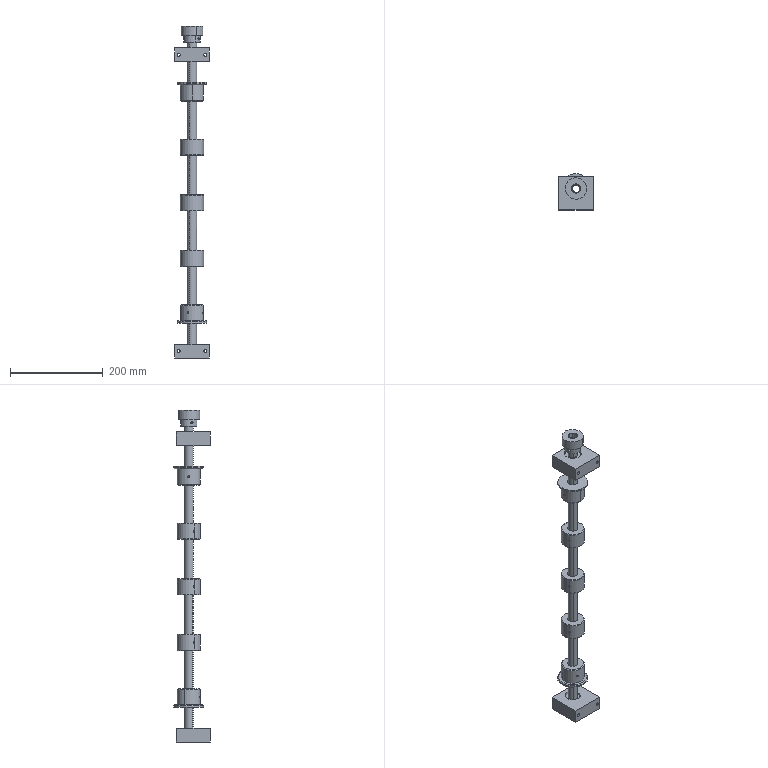Part | SolidWorks | 13 solids | 231 faces | box 74 x 78.5 x 717 mm | volume 691703 mm3 | cylinder 116 | plane 59 | cone 40 | torus 16 | commonest cylinder face diameters 4.2 x28 20 x22 50 x10 6.6 x8 11 x8 37 x8